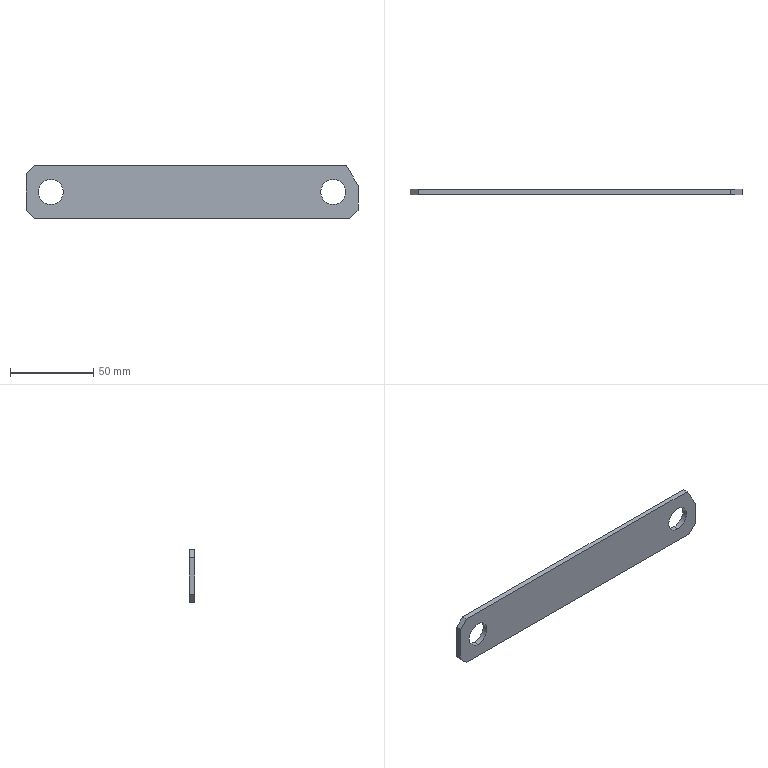Part | SolidWorks | features FlatPattern 1, SMBaseFlange 1, SheetMetal 1 | 1 solid | 14 faces | box 200 x 3.2 x 32 mm | volume 19095 mm3 | plane 10 | cylinder 4 | commonest cylinder face diameters 15 x4
STEP:
#1=CARTESIAN_POINT('',(185.,-3.2,8.5));
#2=VERTEX_POINT('',#1);
#3=CARTESIAN_POINT('',(185.,-3.2,23.5));
#4=VERTEX_POINT('',#3);
#5=CARTESIAN_POINT('',(185.,-3.2,16.));
#6=DIRECTION('',(0.,1.,0.));
#7=DIRECTION('',(0.,0.,1.));
#8=AXIS2_PLACEMENT_3D('',#5,#6,#7);
#9=CIRCLE('',#8,7.5);
#10=EDGE_CURVE('',#2,#4,#9,.T.);
#11=ORIENTED_EDGE('',*,*,#10,.F.);
#12=CARTESIAN_POINT('',(185.,0.,8.5));
#13=VERTEX_POINT('',#12);
#14=CARTESIAN_POINT('',(185.,-3.2,8.5));
#15=DIRECTION('',(0.,1.,0.));
#16=VECTOR('',#15,1000.);
#17=LINE('',#14,#16);
#18=EDGE_CURVE('',#2,#13,#17,.T.);
#19=ORIENTED_EDGE('',*,*,#18,.T.);
#20=CARTESIAN_POINT('',(185.,0.,23.5));
#21=VERTEX_POINT('',#20);
#22=CARTESIAN_POINT('',(185.,0.,16.));
#23=DIRECTION('',(0.,1.,0.));
#24=DIRECTION('',(0.,0.,1.));
#25=AXIS2_PLACEMENT_3D('',#22,#23,#24);
#26=CIRCLE('',#25,7.5);
#27=EDGE_CURVE('',#13,#21,#26,.T.);
#28=ORIENTED_EDGE('',*,*,#27,.T.);
#29=CARTESIAN_POINT('',(185.,-3.2,23.5));
#30=DIRECTION('',(0.,1.,0.));
#31=VECTOR('',#30,1000.);
#32=LINE('',#29,#31);
#33=EDGE_CURVE('',#4,#21,#32,.T.);
#34=ORIENTED_EDGE('',*,*,#33,.F.);
#35=EDGE_LOOP('',(#11,#19,#28,#34));
#36=FACE_OUTER_BOUND('',#35,.T.);
#37=CARTESIAN_POINT('',(185.,-3.2,16.));
#38=DIRECTION('',(0.,1.,0.));
#39=DIRECTION('',(0.,0.,1.));
#40=AXIS2_PLACEMENT_3D('',#37,#38,#39);
#41=CYLINDRICAL_SURFACE('',#40,7.5);
#42=ADVANCED_FACE('',(#36),#41,.F.);
#43=CARTESIAN_POINT('',(15.,-3.2,8.5));
#44=VERTEX_POINT('',#43);
#45=CARTESIAN_POINT('',(15.,-3.2,23.5));
#46=VERTEX_POINT('',#45);
#47=CARTESIAN_POINT('',(15.,-3.2,16.));
#48=DIRECTION('',(0.,1.,0.));
#49=DIRECTION('',(0.,0.,1.));
#50=AXIS2_PLACEMENT_3D('',#47,#48,#49);
#51=CIRCLE('',#50,7.5);
#52=EDGE_CURVE('',#44,#46,#51,.T.);
#53=ORIENTED_EDGE('',*,*,#52,.F.);
#54=CARTESIAN_POINT('',(15.,0.,8.5));
#55=VERTEX_POINT('',#54);
#56=CARTESIAN_POINT('',(15.,-3.2,8.5));
#57=DIRECTION('',(0.,1.,0.));
#58=VECTOR('',#57,1000.);
#59=LINE('',#56,#58);
#60=EDGE_CURVE('',#44,#55,#59,.T.);
#61=ORIENTED_EDGE('',*,*,#60,.T.);
#62=CARTESIAN_POINT('',(15.,0.,23.5));
#63=VERTEX_POINT('',#62);
#64=CARTESIAN_POINT('',(15.,0.,16.));
#65=DIRECTION('',(0.,1.,0.));
#66=DIRECTION('',(0.,0.,1.));
#67=AXIS2_PLACEMENT_3D('',#64,#65,#66);
#68=CIRCLE('',#67,7.5);
#69=EDGE_CURVE('',#55,#63,#68,.T.);
#70=ORIENTED_EDGE('',*,*,#69,.T.);
#71=CARTESIAN_POINT('',(15.,-3.2,23.5));
#72=DIRECTION('',(0.,1.,0.));
#73=VECTOR('',#72,1000.);
#74=LINE('',#71,#73);
#75=EDGE_CURVE('',#46,#63,#74,.T.);
#76=ORIENTED_EDGE('',*,*,#75,.F.);
#77=EDGE_LOOP('',(#53,#61,#70,#76));
#78=FACE_OUTER_BOUND('',#77,.T.);
#79=CARTESIAN_POINT('',(15.,-3.2,16.));
#80=DIRECTION('',(0.,1.,0.));
#81=DIRECTION('',(0.,0.,1.));
#82=AXIS2_PLACEMENT_3D('',#79,#80,#81);
#83=CYLINDRICAL_SURFACE('',#82,7.5);
#84=ADVANCED_FACE('',(#78),#83,.F.);
#85=CARTESIAN_POINT('',(0.,0.,5.));
#86=VERTEX_POINT('',#85);
#87=CARTESIAN_POINT('',(0.,0.,27.));
#88=VERTEX_POINT('',#87);
#89=CARTESIAN_POINT('',(0.,0.,5.));
#90=DIRECTION('',(0.,0.,1.));
#91=VECTOR('',#90,1000.);
#92=LINE('',#89,#91);
#93=EDGE_CURVE('',#86,#88,#92,.T.);
#94=ORIENTED_EDGE('',*,*,#93,.F.);
#95=CARTESIAN_POINT('',(0.,-3.2,5.));
#96=VERTEX_POINT('',#95);
#97=CARTESIAN_POINT('',(0.,-3.2,5.));
#98=DIRECTION('',(0.,1.,0.));
#99=VECTOR('',#98,1000.);
#100=LINE('',#97,#99);
#101=EDGE_CURVE('',#96,#86,#100,.T.);
#102=ORIENTED_EDGE('',*,*,#101,.F.);
#103=CARTESIAN_POINT('',(0.,-3.2,27.));
#104=VERTEX_POINT('',#103);
#105=CARTESIAN_POINT('',(0.,-3.2,5.));
#106=DIRECTION('',(0.,0.,1.));
#107=VECTOR('',#106,1000.);
#108=LINE('',#105,#107);
#109=EDGE_CURVE('',#96,#104,#108,.T.);
#110=ORIENTED_EDGE('',*,*,#109,.T.);
#111=CARTESIAN_POINT('',(0.,-3.2,27.));
#112=DIRECTION('',(0.,1.,0.));
#113=VECTOR('',#112,1000.);
#114=LINE('',#111,#113);
#115=EDGE_CURVE('',#104,#88,#114,.T.);
#116=ORIENTED_EDGE('',*,*,#115,.T.);
#117=EDGE_LOOP('',(#94,#102,#110,#116));
#118=FACE_OUTER_BOUND('',#117,.T.);
#119=CARTESIAN_POINT('',(0.,-3.2,5.));
#120=DIRECTION('',(-1.,0.,0.));
#121=DIRECTION('',(0.,0.,1.));
#122=AXIS2_PLACEMENT_3D('',#119,#120,#121);
#123=PLANE('',#122);
#124=ADVANCED_FACE('',(#118),#123,.T.);
#125=CARTESIAN_POINT('',(5.,0.,0.));
#126=VERTEX_POINT('',#125);
#127=CARTESIAN_POINT('',(0.,0.,5.));
#128=DIRECTION('',(-0.7071,0.,0.7071));
#129=VECTOR('',#128,1000.);
#130=LINE('',#127,#129);
#131=EDGE_CURVE('',#126,#86,#130,.T.);
#132=ORIENTED_EDGE('',*,*,#131,.F.);
#133=CARTESIAN_POINT('',(5.,-3.2,0.));
#134=VERTEX_POINT('',#133);
#135=CARTESIAN_POINT('',(5.,-3.2,0.));
#136=DIRECTION('',(0.,1.,0.));
#137=VECTOR('',#136,1000.);
#138=LINE('',#135,#137);
#139=EDGE_CURVE('',#134,#126,#138,.T.);
#140=ORIENTED_EDGE('',*,*,#139,.F.);
#141=CARTESIAN_POINT('',(0.,-3.2,5.));
#142=DIRECTION('',(-0.7071,0.,0.7071));
#143=VECTOR('',#142,1000.);
#144=LINE('',#141,#143);
#145=EDGE_CURVE('',#134,#96,#144,.T.);
#146=ORIENTED_EDGE('',*,*,#145,.T.);
#147=ORIENTED_EDGE('',*,*,#101,.T.);
#148=EDGE_LOOP('',(#132,#140,#146,#147));
#149=FACE_OUTER_BOUND('',#148,.T.);
#150=CARTESIAN_POINT('',(0.,-3.2,5.));
#151=DIRECTION('',(-0.7071,0.,-0.7071));
#152=DIRECTION('',(-0.7071,0.,0.7071));
#153=AXIS2_PLACEMENT_3D('',#150,#151,#152);
#154=PLANE('',#153);
#155=ADVANCED_FACE('',(#149),#154,.T.);
#156=CARTESIAN_POINT('',(195.,0.,0.));
#157=VERTEX_POINT('',#156);
#158=CARTESIAN_POINT('',(5.,0.,0.));
#159=DIRECTION('',(-1.,0.,0.));
#160=VECTOR('',#159,1000.);
#161=LINE('',#158,#160);
#162=EDGE_CURVE('',#157,#126,#161,.T.);
#163=ORIENTED_EDGE('',*,*,#162,.F.);
#164=CARTESIAN_POINT('',(195.,-3.2,0.));
#165=VERTEX_POINT('',#164);
#166=CARTESIAN_POINT('',(195.,-3.2,0.));
#167=DIRECTION('',(0.,1.,0.));
#168=VECTOR('',#167,1000.);
#169=LINE('',#166,#168);
#170=EDGE_CURVE('',#165,#157,#169,.T.);
#171=ORIENTED_EDGE('',*,*,#170,.F.);
#172=CARTESIAN_POINT('',(5.,-3.2,0.));
#173=DIRECTION('',(-1.,0.,0.));
#174=VECTOR('',#173,1000.);
#175=LINE('',#172,#174);
#176=EDGE_CURVE('',#165,#134,#175,.T.);
#177=ORIENTED_EDGE('',*,*,#176,.T.);
#178=ORIENTED_EDGE('',*,*,#139,.T.);
#179=EDGE_LOOP('',(#163,#171,#177,#178));
#180=FACE_OUTER_BOUND('',#179,.T.);
#181=CARTESIAN_POINT('',(5.,-3.2,0.));
#182=DIRECTION('',(0.,0.,-1.));
#183=DIRECTION('',(-1.,0.,0.));
#184=AXIS2_PLACEMENT_3D('',#181,#182,#183);
#185=PLANE('',#184);
#186=ADVANCED_FACE('',(#180),#185,.T.);
#187=CARTESIAN_POINT('',(200.,0.,5.));
#188=VERTEX_POINT('',#187);
#189=CARTESIAN_POINT('',(195.,0.,0.));
#190=DIRECTION('',(-0.7071,0.,-0.7071));
#191=VECTOR('',#190,1000.);
#192=LINE('',#189,#191);
#193=EDGE_CURVE('',#188,#157,#192,.T.);
#194=ORIENTED_EDGE('',*,*,#193,.F.);
#195=CARTESIAN_POINT('',(200.,-3.2,5.));
#196=VERTEX_POINT('',#195);
#197=CARTESIAN_POINT('',(200.,-3.2,5.));
#198=DIRECTION('',(0.,1.,0.));
#199=VECTOR('',#198,1000.);
#200=LINE('',#197,#199);
#201=EDGE_CURVE('',#196,#188,#200,.T.);
#202=ORIENTED_EDGE('',*,*,#201,.F.);
#203=CARTESIAN_POINT('',(195.,-3.2,0.));
#204=DIRECTION('',(-0.7071,0.,-0.7071));
#205=VECTOR('',#204,1000.);
#206=LINE('',#203,#205);
#207=EDGE_CURVE('',#196,#165,#206,.T.);
#208=ORIENTED_EDGE('',*,*,#207,.T.);
#209=ORIENTED_EDGE('',*,*,#170,.T.);
#210=EDGE_LOOP('',(#194,#202,#208,#209));
#211=FACE_OUTER_BOUND('',#210,.T.);
#212=CARTESIAN_POINT('',(195.,-3.2,0.));
#213=DIRECTION('',(0.7071,0.,-0.7071));
#214=DIRECTION('',(-0.7071,0.,-0.7071));
#215=AXIS2_PLACEMENT_3D('',#212,#213,#214);
#216=PLANE('',#215);
#217=ADVANCED_FACE('',(#211),#216,.T.);
#218=CARTESIAN_POINT('',(200.,0.,20.));
#219=VERTEX_POINT('',#218);
#220=CARTESIAN_POINT('',(200.,0.,5.));
#221=DIRECTION('',(0.,0.,-1.));
#222=VECTOR('',#221,1000.);
#223=LINE('',#220,#222);
#224=EDGE_CURVE('',#219,#188,#223,.T.);
#225=ORIENTED_EDGE('',*,*,#224,.F.);
#226=CARTESIAN_POINT('',(200.,-3.2,20.));
#227=VERTEX_POINT('',#226);
#228=CARTESIAN_POINT('',(200.,-3.2,20.));
#229=DIRECTION('',(0.,1.,0.));
#230=VECTOR('',#229,1000.);
#231=LINE('',#228,#230);
#232=EDGE_CURVE('',#227,#219,#231,.T.);
#233=ORIENTED_EDGE('',*,*,#232,.F.);
#234=CARTESIAN_POINT('',(200.,-3.2,5.));
#235=DIRECTION('',(0.,0.,-1.));
#236=VECTOR('',#235,1000.);
#237=LINE('',#234,#236);
#238=EDGE_CURVE('',#227,#196,#237,.T.);
#239=ORIENTED_EDGE('',*,*,#238,.T.);
#240=ORIENTED_EDGE('',*,*,#201,.T.);
#241=EDGE_LOOP('',(#225,#233,#239,#240));
#242=FACE_OUTER_BOUND('',#241,.T.);
#243=CARTESIAN_POINT('',(200.,-3.2,5.));
#244=DIRECTION('',(1.,0.,0.));
#245=DIRECTION('',(0.,0.,-1.));
#246=AXIS2_PLACEMENT_3D('',#243,#244,#245);
#247=PLANE('',#246);
#248=ADVANCED_FACE('',(#242),#247,.T.);
#249=CARTESIAN_POINT('',(193.,0.,32.));
#250=VERTEX_POINT('',#249);
#251=CARTESIAN_POINT('',(193.,0.,32.));
#252=DIRECTION('',(0.5039,0.,-0.8638));
#253=VECTOR('',#252,1000.);
#254=LINE('',#251,#253);
#255=EDGE_CURVE('',#250,#219,#254,.T.);
#256=ORIENTED_EDGE('',*,*,#255,.F.);
#257=CARTESIAN_POINT('',(193.,-3.2,32.));
#258=VERTEX_POINT('',#257);
#259=CARTESIAN_POINT('',(193.,-3.2,32.));
#260=DIRECTION('',(0.,1.,0.));
#261=VECTOR('',#260,1000.);
#262=LINE('',#259,#261);
#263=EDGE_CURVE('',#258,#250,#262,.T.);
#264=ORIENTED_EDGE('',*,*,#263,.F.);
#265=CARTESIAN_POINT('',(193.,-3.2,32.));
#266=DIRECTION('',(0.5039,0.,-0.8638));
#267=VECTOR('',#266,1000.);
#268=LINE('',#265,#267);
#269=EDGE_CURVE('',#258,#227,#268,.T.);
#270=ORIENTED_EDGE('',*,*,#269,.T.);
#271=ORIENTED_EDGE('',*,*,#232,.T.);
#272=EDGE_LOOP('',(#256,#264,#270,#271));
#273=FACE_OUTER_BOUND('',#272,.T.);
#274=CARTESIAN_POINT('',(193.,-3.2,32.));
#275=DIRECTION('',(0.8638,0.,0.5039));
#276=DIRECTION('',(0.5039,0.,-0.8638));
#277=AXIS2_PLACEMENT_3D('',#274,#275,#276);
#278=PLANE('',#277);
#279=ADVANCED_FACE('',(#273),#278,.T.);
#280=CARTESIAN_POINT('',(5.,0.,32.));
#281=VERTEX_POINT('',#280);
#282=CARTESIAN_POINT('',(5.,0.,32.));
#283=DIRECTION('',(1.,0.,0.));
#284=VECTOR('',#283,1000.);
#285=LINE('',#282,#284);
#286=EDGE_CURVE('',#281,#250,#285,.T.);
#287=ORIENTED_EDGE('',*,*,#286,.F.);
#288=CARTESIAN_POINT('',(5.,-3.2,32.));
#289=VERTEX_POINT('',#288);
#290=CARTESIAN_POINT('',(5.,-3.2,32.));
#291=DIRECTION('',(0.,1.,0.));
#292=VECTOR('',#291,1000.);
#293=LINE('',#290,#292);
#294=EDGE_CURVE('',#289,#281,#293,.T.);
#295=ORIENTED_EDGE('',*,*,#294,.F.);
#296=CARTESIAN_POINT('',(5.,-3.2,32.));
#297=DIRECTION('',(1.,0.,0.));
#298=VECTOR('',#297,1000.);
#299=LINE('',#296,#298);
#300=EDGE_CURVE('',#289,#258,#299,.T.);
#301=ORIENTED_EDGE('',*,*,#300,.T.);
#302=ORIENTED_EDGE('',*,*,#263,.T.);
#303=EDGE_LOOP('',(#287,#295,#301,#302));
#304=FACE_OUTER_BOUND('',#303,.T.);
#305=CARTESIAN_POINT('',(5.,-3.2,32.));
#306=DIRECTION('',(0.,0.,1.));
#307=DIRECTION('',(1.,0.,0.));
#308=AXIS2_PLACEMENT_3D('',#305,#306,#307);
#309=PLANE('',#308);
#310=ADVANCED_FACE('',(#304),#309,.T.);
#311=CARTESIAN_POINT('',(0.,0.,27.));
#312=DIRECTION('',(0.7071,0.,0.7071));
#313=VECTOR('',#312,1000.);
#314=LINE('',#311,#313);
#315=EDGE_CURVE('',#88,#281,#314,.T.);
#316=ORIENTED_EDGE('',*,*,#315,.F.);
#317=ORIENTED_EDGE('',*,*,#115,.F.);
#318=CARTESIAN_POINT('',(0.,-3.2,27.));
#319=DIRECTION('',(0.7071,0.,0.7071));
#320=VECTOR('',#319,1000.);
#321=LINE('',#318,#320);
#322=EDGE_CURVE('',#104,#289,#321,.T.);
#323=ORIENTED_EDGE('',*,*,#322,.T.);
#324=ORIENTED_EDGE('',*,*,#294,.T.);
#325=EDGE_LOOP('',(#316,#317,#323,#324));
#326=FACE_OUTER_BOUND('',#325,.T.);
#327=CARTESIAN_POINT('',(0.,-3.2,27.));
#328=DIRECTION('',(-0.7071,0.,0.7071));
#329=DIRECTION('',(0.7071,0.,0.7071));
#330=AXIS2_PLACEMENT_3D('',#327,#328,#329);
#331=PLANE('',#330);
#332=ADVANCED_FACE('',(#326),#331,.T.);
#333=CARTESIAN_POINT('',(185.,-3.2,16.));
#334=DIRECTION('',(0.,1.,0.));
#335=DIRECTION('',(0.,0.,1.));
#336=AXIS2_PLACEMENT_3D('',#333,#334,#335);
#337=CIRCLE('',#336,7.5);
#338=EDGE_CURVE('',#4,#2,#337,.T.);
#339=ORIENTED_EDGE('',*,*,#338,.T.);
#340=ORIENTED_EDGE('',*,*,#10,.T.);
#341=EDGE_LOOP('',(#339,#340));
#342=FACE_BOUND('',#341,.T.);
#343=CARTESIAN_POINT('',(15.,-3.2,16.));
#344=DIRECTION('',(0.,1.,0.));
#345=DIRECTION('',(0.,0.,1.));
#346=AXIS2_PLACEMENT_3D('',#343,#344,#345);
#347=CIRCLE('',#346,7.5);
#348=EDGE_CURVE('',#46,#44,#347,.T.);
#349=ORIENTED_EDGE('',*,*,#348,.T.);
#350=ORIENTED_EDGE('',*,*,#52,.T.);
#351=EDGE_LOOP('',(#349,#350));
#352=FACE_BOUND('',#351,.T.);
#353=ORIENTED_EDGE('',*,*,#109,.F.);
#354=ORIENTED_EDGE('',*,*,#145,.F.);
#355=ORIENTED_EDGE('',*,*,#176,.F.);
#356=ORIENTED_EDGE('',*,*,#207,.F.);
#357=ORIENTED_EDGE('',*,*,#238,.F.);
#358=ORIENTED_EDGE('',*,*,#269,.F.);
#359=ORIENTED_EDGE('',*,*,#300,.F.);
#360=ORIENTED_EDGE('',*,*,#322,.F.);
#361=EDGE_LOOP('',(#353,#354,#355,#356,#357,#358,#359,#360));
#362=FACE_OUTER_BOUND('',#361,.T.);
#363=CARTESIAN_POINT('',(0.,-3.2,0.));
#364=DIRECTION('',(0.,1.,0.));
#365=DIRECTION('',(0.,0.,1.));
#366=AXIS2_PLACEMENT_3D('',#363,#364,#365);
#367=PLANE('',#366);
#368=ADVANCED_FACE('',(#342,#352,#362),#367,.F.);
#369=CARTESIAN_POINT('',(185.,0.,16.));
#370=DIRECTION('',(0.,1.,0.));
#371=DIRECTION('',(0.,0.,1.));
#372=AXIS2_PLACEMENT_3D('',#369,#370,#371);
#373=CIRCLE('',#372,7.5);
#374=EDGE_CURVE('',#21,#13,#373,.T.);
#375=ORIENTED_EDGE('',*,*,#374,.F.);
#376=ORIENTED_EDGE('',*,*,#27,.F.);
#377=EDGE_LOOP('',(#375,#376));
#378=FACE_BOUND('',#377,.T.);
#379=CARTESIAN_POINT('',(15.,0.,16.));
#380=DIRECTION('',(0.,1.,0.));
#381=DIRECTION('',(0.,0.,1.));
#382=AXIS2_PLACEMENT_3D('',#379,#380,#381);
#383=CIRCLE('',#382,7.5);
#384=EDGE_CURVE('',#63,#55,#383,.T.);
#385=ORIENTED_EDGE('',*,*,#384,.F.);
#386=ORIENTED_EDGE('',*,*,#69,.F.);
#387=EDGE_LOOP('',(#385,#386));
#388=FACE_BOUND('',#387,.T.);
#389=ORIENTED_EDGE('',*,*,#93,.T.);
#390=ORIENTED_EDGE('',*,*,#315,.T.);
#391=ORIENTED_EDGE('',*,*,#286,.T.);
#392=ORIENTED_EDGE('',*,*,#255,.T.);
#393=ORIENTED_EDGE('',*,*,#224,.T.);
#394=ORIENTED_EDGE('',*,*,#193,.T.);
#395=ORIENTED_EDGE('',*,*,#162,.T.);
#396=ORIENTED_EDGE('',*,*,#131,.T.);
#397=EDGE_LOOP('',(#389,#390,#391,#392,#393,#394,#395,#396));
#398=FACE_OUTER_BOUND('',#397,.T.);
#399=CARTESIAN_POINT('',(0.,0.,0.));
#400=DIRECTION('',(0.,1.,0.));
#401=DIRECTION('',(0.,0.,1.));
#402=AXIS2_PLACEMENT_3D('',#399,#400,#401);
#403=PLANE('',#402);
#404=ADVANCED_FACE('',(#378,#388,#398),#403,.T.);
#405=ORIENTED_EDGE('',*,*,#60,.F.);
#406=ORIENTED_EDGE('',*,*,#348,.F.);
#407=ORIENTED_EDGE('',*,*,#75,.T.);
#408=ORIENTED_EDGE('',*,*,#384,.T.);
#409=EDGE_LOOP('',(#405,#406,#407,#408));
#410=FACE_OUTER_BOUND('',#409,.T.);
#411=CARTESIAN_POINT('',(15.,-3.2,16.));
#412=DIRECTION('',(0.,1.,0.));
#413=DIRECTION('',(0.,0.,1.));
#414=AXIS2_PLACEMENT_3D('',#411,#412,#413);
#415=CYLINDRICAL_SURFACE('',#414,7.5);
#416=ADVANCED_FACE('',(#410),#415,.F.);
#417=ORIENTED_EDGE('',*,*,#18,.F.);
#418=ORIENTED_EDGE('',*,*,#338,.F.);
#419=ORIENTED_EDGE('',*,*,#33,.T.);
#420=ORIENTED_EDGE('',*,*,#374,.T.);
#421=EDGE_LOOP('',(#417,#418,#419,#420));
#422=FACE_OUTER_BOUND('',#421,.T.);
#423=CARTESIAN_POINT('',(185.,-3.2,16.));
#424=DIRECTION('',(0.,1.,0.));
#425=DIRECTION('',(0.,0.,1.));
#426=AXIS2_PLACEMENT_3D('',#423,#424,#425);
#427=CYLINDRICAL_SURFACE('',#426,7.5);
#428=ADVANCED_FACE('',(#422),#427,.F.);
#429=CLOSED_SHELL('',(#42,#84,#124,#155,#186,#217,#248,#279,#310,#332,#368,#404,#416,#428));
#430=MANIFOLD_SOLID_BREP('',#429);
#431=CARTESIAN_POINT('',(0.,0.,0.));
#432=DIRECTION('',(0.,0.,1.));
#433=DIRECTION('',(1.,0.,0.));
#434=AXIS2_PLACEMENT_3D('',#431,#432,#433);
#435=(LENGTH_UNIT()NAMED_UNIT(*)SI_UNIT(.MILLI.,.METRE.));
#436=UNCERTAINTY_MEASURE_WITH_UNIT(LENGTH_MEASURE(0.00001),#435,'','');
#437=(NAMED_UNIT(*)PLANE_ANGLE_UNIT()SI_UNIT($,.RADIAN.));
#438=(NAMED_UNIT(*)SI_UNIT($,.STERADIAN.)SOLID_ANGLE_UNIT());
#439=(GEOMETRIC_REPRESENTATION_CONTEXT(3)GLOBAL_UNCERTAINTY_ASSIGNED_CONTEXT((#436))GLOBAL_UNIT_ASSIGNED_CONTEXT((#435,#437,#438))REPRESENTATION_CONTEXT('',''));
#440=ADVANCED_BREP_SHAPE_REPRESENTATION('',(#430,#434),#439);